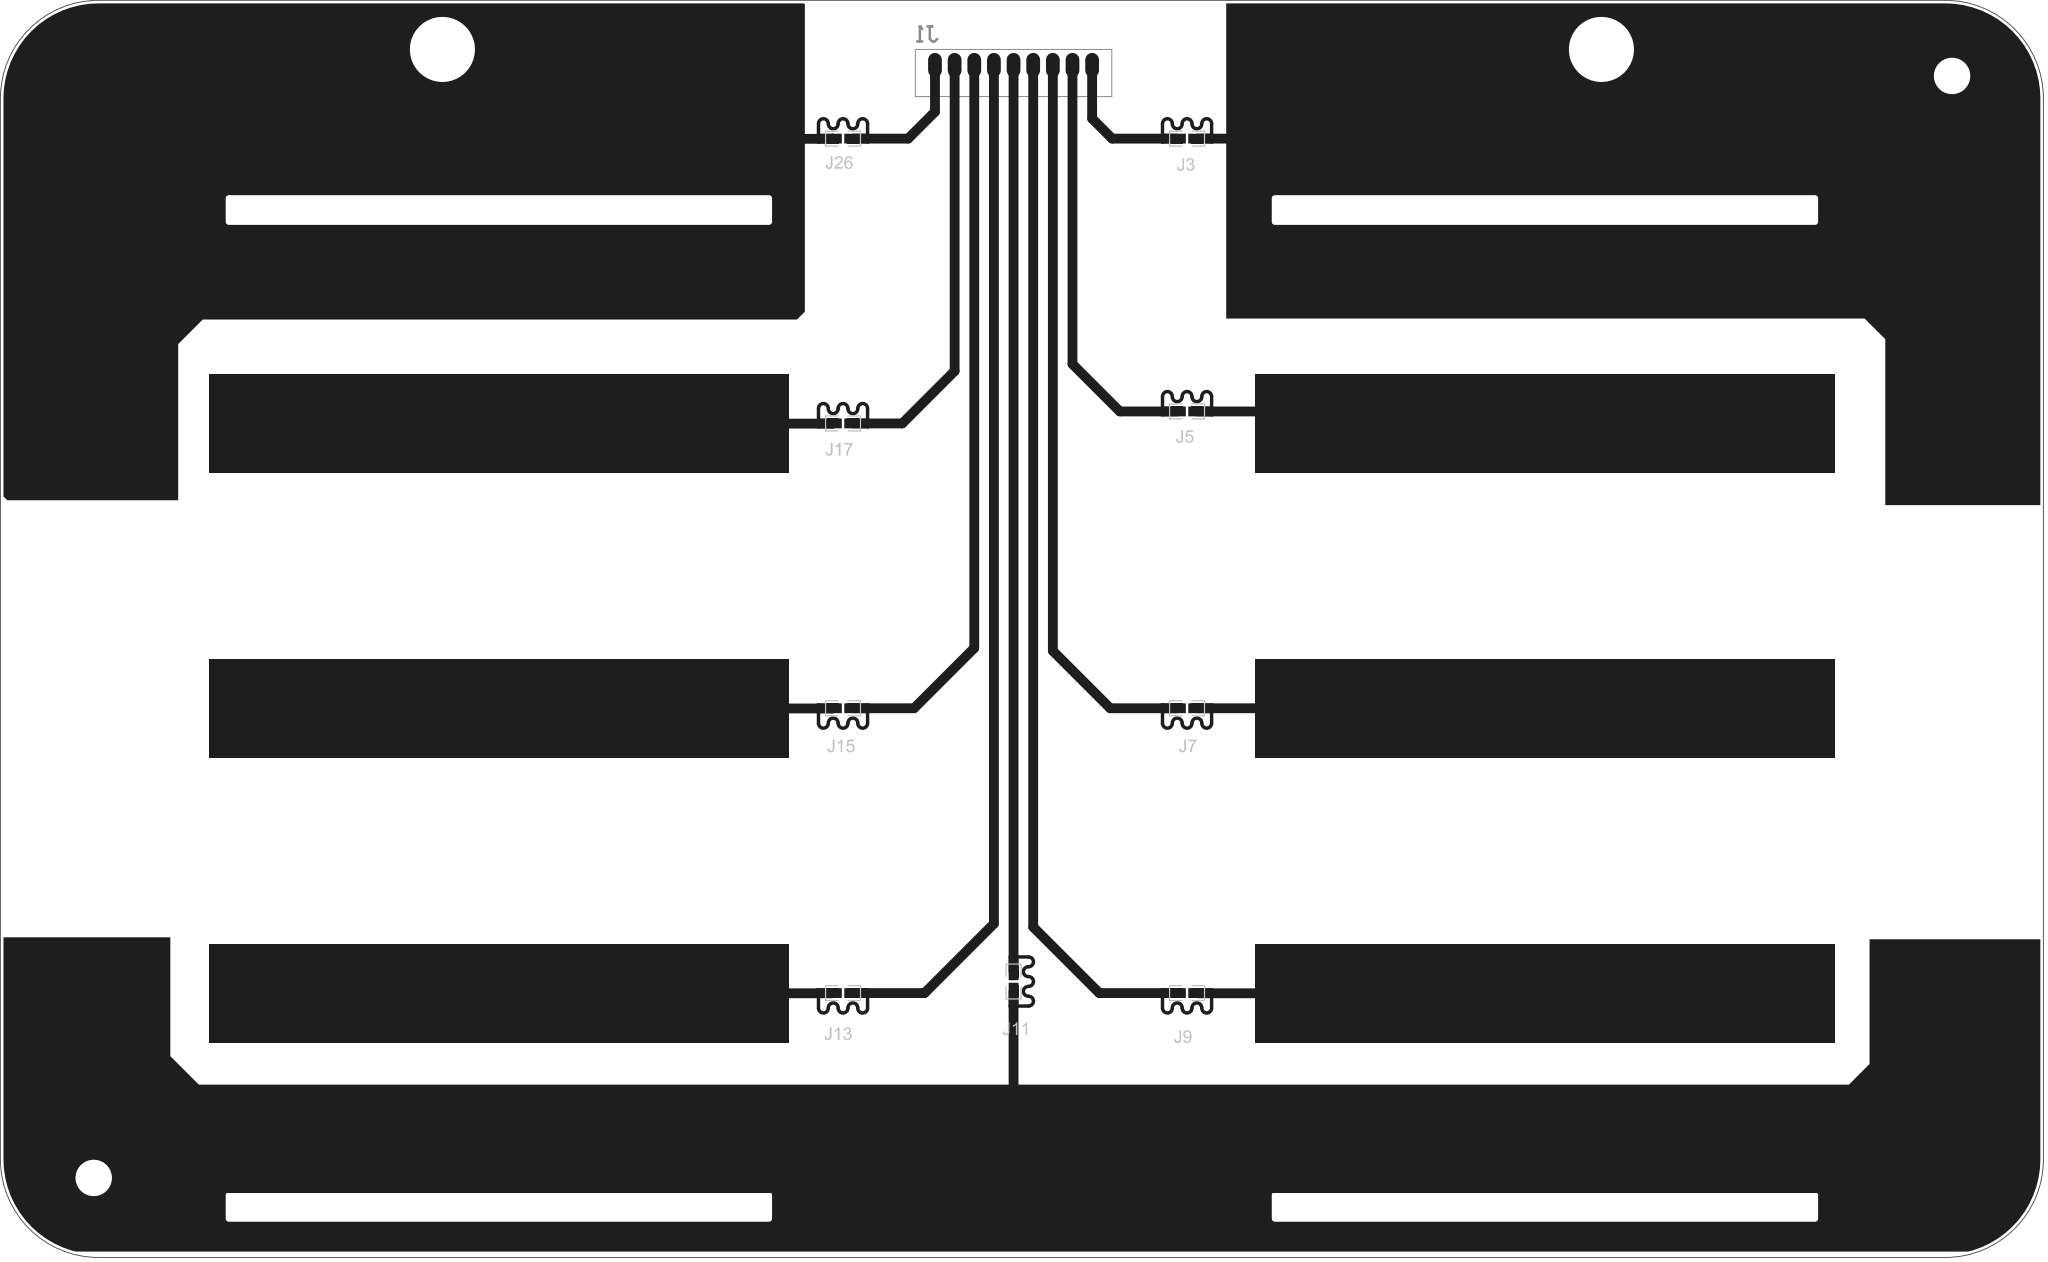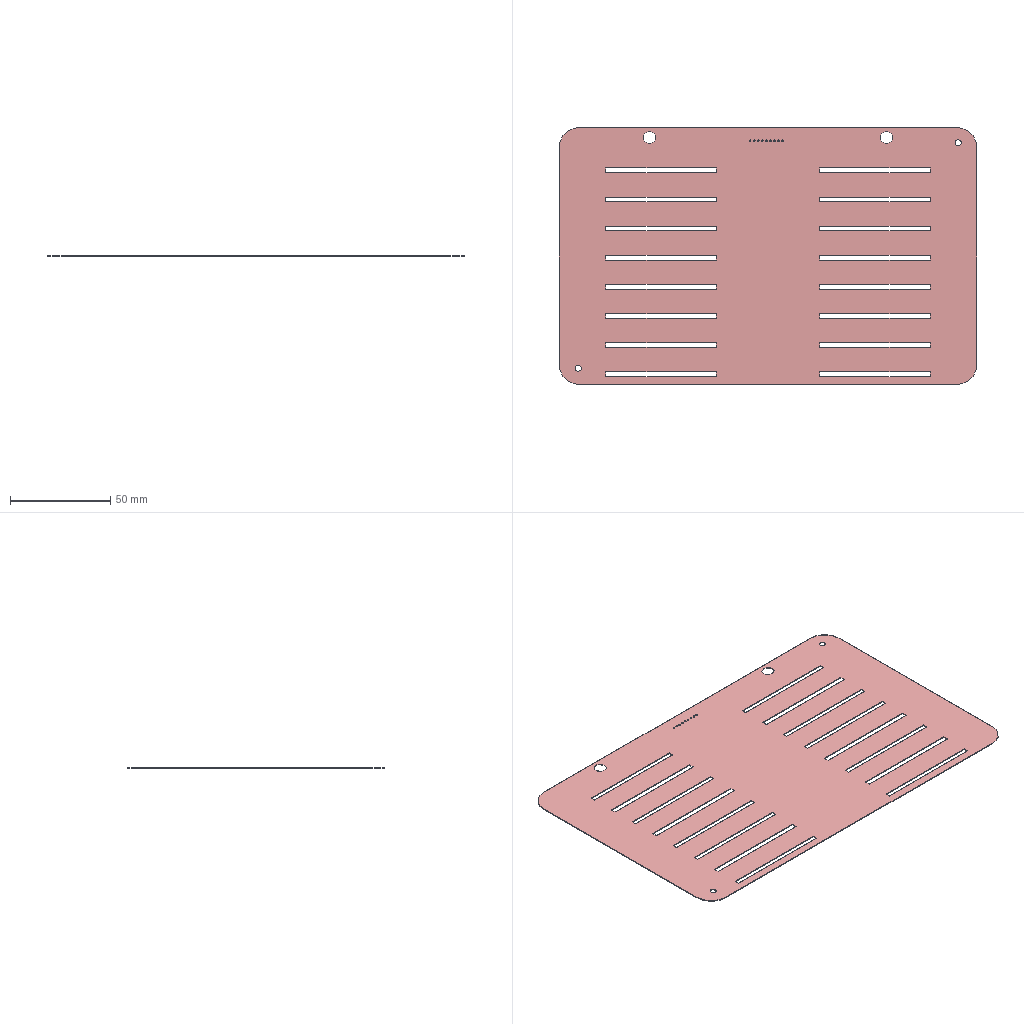Circuit board layout | Altium Designer | box 208 x 128 x 0.4 mm
Layer stack:
# Altium Designer layer stack of  (unit mm; dielectric type: 0 none, 1 core, 2 prepreg, 3 surface material)
index,name,kind,layer,copper_thickness_mm,dielectric_type,dielectric_thickness_mm,dielectric_material,dielectric_constant
0,Top Paste,other,,,,,,
1,Top Overlay,other,,,,,,
2,Top Solder,dielectric,,,3,0.0102,Solder Resist,3.5
3,Top Layer,copper,Top Layer,0.0356,,,,
4,Dielectric 1,dielectric,,,0,0.32,FR-4,4.8
5,Bottom Layer,copper,Bottom Layer,0.0356,,,,
6,Bottom Solder,dielectric,,,3,0.0102,Solder Resist,3.5
7,Bottom Overlay,other,,,,,,
8,Bottom Paste,other,,,,,,
# drill layer pairs: low layer,high layer
drill_pair,Top Layer,Bottom Layer
Part placement:
Designator,Comment,Layer,Footprint,Center-X(mm),Center-Y(mm),Rotation
J1,HX-2.54mm-9P through-hole connector with latch,BottomLayer,HX2.0-9P,93.15,3.4,180
B-,Pth,TopLayer,55*10*1MM,147.25,-4.1,180
B+,Pth,TopLayer,55*10*1MM,40.75,-4.1,180
B14,Pth,TopLayer,55*10*1MM,40.75,-33.1,180
B12,Pth,TopLayer,55*10*1MM,40.75,-62.1,180
B10,Pth,TopLayer,55*10*1MM,40.75,-91.1,180
B8,Pth,TopLayer,161.5*10*1MM,94,-106.65,180
B6,Pth,TopLayer,55*10*1MM,147.25,-91.1,180
B4,Pth,TopLayer,55*10*1MM,147.25,-62.1,180
B2,Pth,TopLayer,55*10*1MM,147.25,-33.1,180
J26,FPC,TopLayer,异形电阻,75.789,-4.08,90
J17,FPC,TopLayer,异形电阻,75.789,-33.081,90
J15,FPC,TopLayer,异形电阻,75.789,-62.081,270
J13,FPC,TopLayer,异形电阻,75.789,-91.081,270
J11,FPC,TopLayer,异形电阻,93.15,-89.899,0
J9,FPC,TopLayer,异形电阻,110.814,-91.081,270
J7,FPC,TopLayer,异形电阻,110.814,-62.081,270
J5,FPC,TopLayer,异形电阻,110.814,-31.859,90
J3,FPC,TopLayer,异形电阻,110.814,-4.08,90
Pad and via stacks:
# Altium Designer via and pad stacks of  (unit mm). Each distinct definition once, with the count of objects using it.
# via: kind,start_layer,end_layer,hole_mm,diameter_mm,mode(0 simple;1 top-mid-bottom;2 full stack),diameter_per_layer,count,example_net
# pad: kind,layer,hole_mm,hole_type(0 round;1 square;2 slot),plating,top_size,top_shape(1 round;2 rect;3 octagon;9 rounded rect),mid_size,bottom_size,mode,footprint,size_per_layer,count,example
pad,Top Layer,0,0,plated,1.2x1,2,1.2x1,1.2x1,0,\u00D2\u00EC\u00D0\u00CE\u00B5\u00E7\u00D7\u00E8,,18,J26.2
pad,Top Layer,0,2,plated,1x1,2,1x1,1x1,0,161.5*10*1MM,,1,B8.1
pad,Top Layer,0,2,plated,1x1,2,1x1,1x1,0,55*10*1MM,,8,B-.1
pad,Top Layer,0,0,plated,1.4x2.5,1,1.4x2.5,1.4x2.5,0,HX2.0-9P,,9,J1.1
pad,Top Layer,0,0,plated,1x1,1,1x1,1x1,0,,,2,3
pad,Multi-Layer,0.75,0,plated,0.75x0.75,1,0.75x0.75,0.75x0.75,0,HX2.0-9P,,9,J1.1
Copper pours:
name,layer,net,type(0 solid;1 hatched;2 none)
NONET_L02_P-001,Top Layer,B-,0
NONET_L02_P-001,Top Layer,B+,0
NONET_L02_P-001,Top Layer,B8,0
Design rules, without the lines most boards share:
# Altium Designer design rules of  (exported by Altium Designer, unit mm)
# columns: name | kind | enabled | priority | scope1 | scope2 | descriptor | typed fields (field=value)
NetAntennae | 56 | enabled | 1 | All | All | Net Antennae (Tolerance=0mm) (All) |
SilkToSilkClearance | 55 | enabled | 1 | All | All | Silk to Silk (Clearance=0mm) (All),(All) |
SilkToSolderMaskClearance | 54 | enabled | 1 | IsPad | All | Silk To Solder Mask (Clearance=0mm) (IsPad),(All) |
MinimumSolderMaskSliver | 53 | enabled | 1 | All | All | Minimum Solder Mask Sliver (Gap=0mm) (All),(All) |
HoleToHoleClearance | 52 | enabled | 1 | All | All | Hole To Hole Clearance (Gap=0mm) (All),(All) | gap=0
DiffPairsRouting | 51 | enabled | 1 | All | All | Differential Pairs Uncoupled Length using the Gap Constraints (Min=0.254mm) (Max=0.254mm) (Prefered=0.254mm)  and Width Constraints (Min=0.381mm) (Max=0.381mm) (Prefered=0.381mm) (All) |
HoleSize | 42 | enabled | 1 | All | All | Hole Size Constraint (Min=0.025mm) (Max=2.54mm) (All) |
Height | 50 | enabled | 1 | All | All | Height Constraint (Min=0mm) (Max=25.4mm) (Prefered=12.7mm) (All) | min_height=0 max_height=25.4
ComponentClearance | 24 | enabled | 1 | All | All | Component Clearance Constraint ( Horizontal Gap = 0mm, Vertical Gap = 0mm ) (All),(All)  | gap=0
SolderMaskExpansion | 13 | enabled | 1 | All | All | Solder Mask Expansion (Expansion =0.102mm) (All) | expansion=0.1016
PasteMaskExpansion | 14 | enabled | 1 | All | All | Paste Mask Expansion (Expansion =0mm) (All) | expansion=0
RoutingVias | 11 | enabled | 1 | All | All | Routing Via (MinHoleWidth=0.711mm) (MaxHoleWidth=0.711mm) (PreferredHoleWidth=0.711mm) (MinWidth=1.27mm) (MaxWidth=1.27mm) (PreferedWidth=1.27mm) (All) | via_min_hole=0.7112 via_max_hole=0.7112 via_preferred_diameter=1.27 via_preferred_hole=0.7112
RoutingCorners | 10 | enabled | 1 | All | All | Routing Corners (Style=45-Degree) (Min Setback=2.54mm) (Max Setback=2.54mm) (All) |
Width | 2 | enabled | 1 | All | All | Width Constraint (Min=0.254mm) (Max=2mm) (Preferred=0.254mm) (All) |
PolygonConnect | 20 | enabled | 1 | All | All | Polygon Connect Rule(Direct Connect )(Conductor Width=0.254mm) (Relief Angle=90 Angle) (Entries=4) (Air Gap Width=0.254mm) (All),(All) | connect_style(0=relief,1=direct,2=none)=1 relief_conductor_width=0.254 relief_entries=4
PlaneClearance | 12 | enabled | 1 | All | All | Power Plane Clearance (Clearance =0.508mm) (All) | clearance=0.508
PlaneConnect | 6 | enabled | 1 | All | All | Power Plane Connect Rule(Relief Connect )(Expansion=0.508mm) (Conductor Width=0.254mm) (Air Gap=0.254mm) (Entries=4) (All) | relief_conductor_width=0.254 relief_entries=4 relief_expansion=0.508
Clearance | 0 | enabled | 1 | All | All | Clearance Constraint (Gap=0.3mm) (All),(All) | gap=0.3
Classes set for this board:
# Altium Designer classes of  (member kind: 0 net, 1 component, 2 from-to, 3 pad, 4 layer, 5 differential pair, 6 design channel, 7 polygon, 8 structure, 9 xSignal)
# columns: class name | member kind | superclass | members
B-TRAN-MD28 V0 | 1 | no | J3; J5; J7; J9; J11; J13; J15; J17; J26; J3; J5; J7; J9; J11; J13; J15; J17; J26; B2; B4; B6; B8; B10; B12; B14; B+; B-; J1;